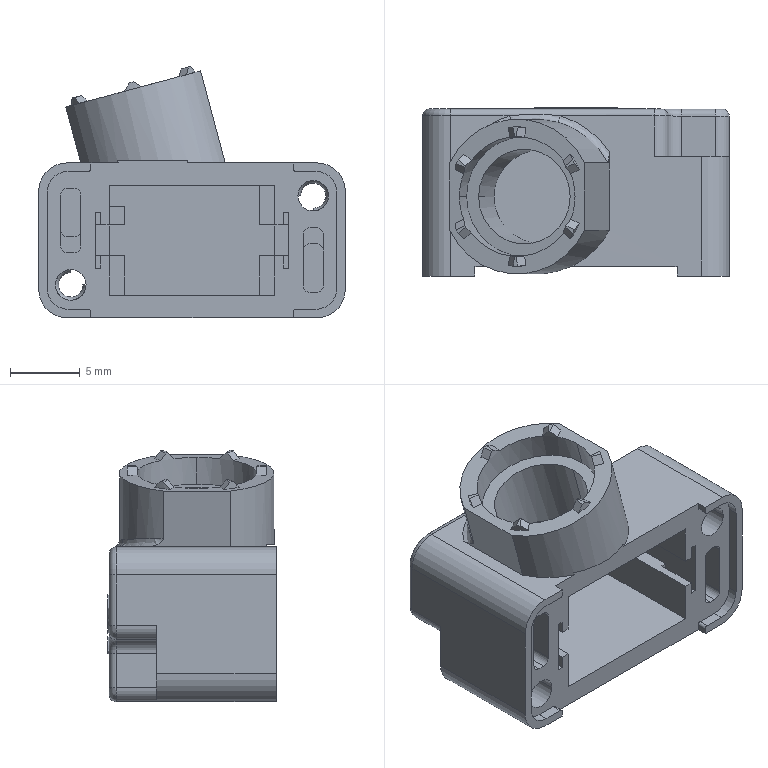Part | STEP file | _1-SO-516090001^MS1H1-40B30CB-A331Z_1_ASM_Motor mount assembly | 1 solid | 310 faces | box 22 x 12.1 x 18.036 mm | volume 1625 mm3 | plane 143 | spline 98 | cylinder 59 | torus 10 | commonest cylinder face diameters 1 x20 2.2 x8 2 x6 10 x6 0.4 x4 3 x4